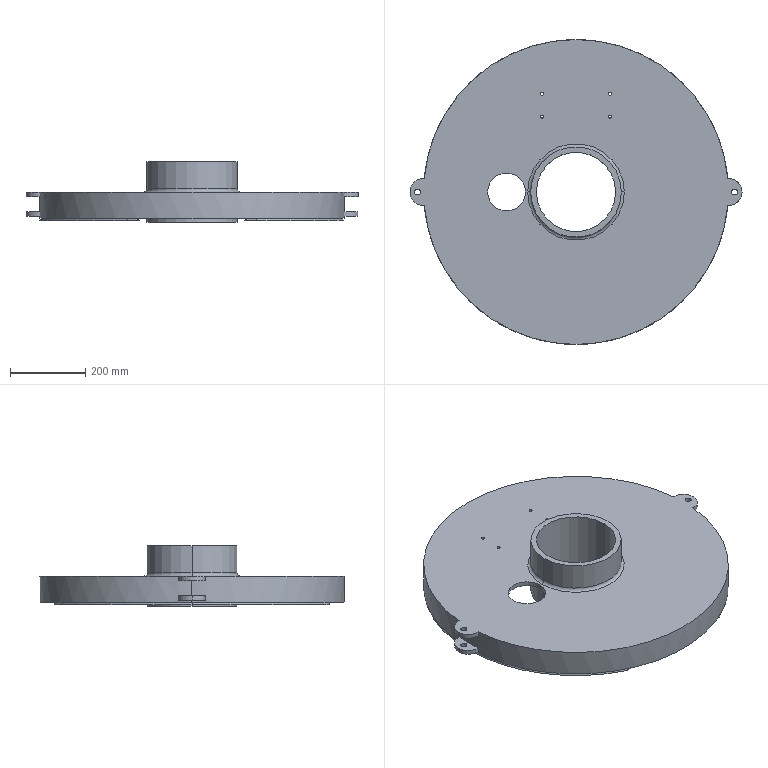Part | NX | features BREP 1 | 1 solid | 61 faces | box 880 x 808 x 160 mm | volume 9751568 mm3 | cylinder 34 | plane 17 | cone 6 | torus 4 | commonest cylinder face diameters 8 x8 16 x8 72 x6 240 x4 100 x2 210 x2